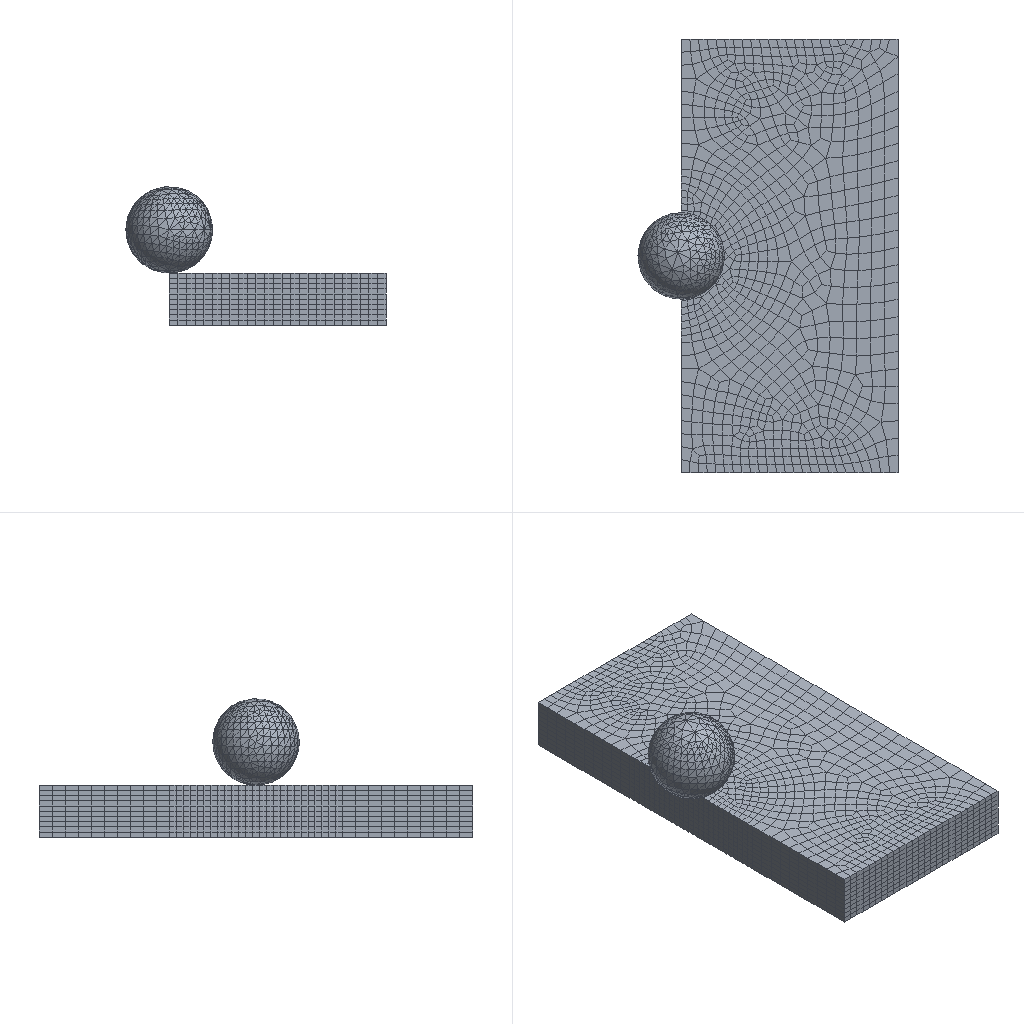Simulation study | abaqus
Set-up summary:
category,name,step,type,value,unit,region
solver,abaqus,,Abaqus/CAE 2024
units,SI m-kg-s (Pa),,inferred,E=2.078e+11 density=7800
analysis,Step-1,,dynamic explicit,nlgeom=True; time_period=4e-05
mesh,nodes,,,11335
mesh,elements,,,13296
element_type,C3D8R,,,8810
element_type,C3D4,,,4486
material,Mat-plate,,E,2.078e+11
material,Mat-plate,,nu,0.3
material,Mat-plate,,density,7800
material,Mat-plate,,yield,1.22e+09
material,Mat-plate,,behaviors,plastic; shear failure
material,Mat_ball,,E,2.09e+11
material,Mat_ball,,nu,0.3
material,Mat_ball,,density,7800
section,Mat_ball,,solid section,,,_PickedSet2
section,Mat-plate,,solid section,,,_PickedSet2
load,velocity,initial,initial condition velocity
bc,BC-plate,initial,fixed,"[dofs=rx,ry,rz,x,y,z n=6]",,_PickedSet11
bc,Symm-plate,initial,ysymm,[dofs=YSYMM],,_PickedSet12
contact,ball-plate,Step-1,contact pair,interaction=contact,,_PickedSurf9 / _PickedSet10_CNS_
constraint,rigid body,,,1
Abaqus input file, long lists of numbers shortened:
*Heading
** Job name: deck Model name: Model-1
** Generated by: Abaqus/CAE 2024
*Preprint, echo=NO, model=NO, history=NO, contact=NO
**
** PARTS
**
*Part, name=Ball
*Node
      1, 0.01545,  0.04755,           0.
      2, 0.02939, 0.04045,           0.
** (970 more lines like these left out)
*Element, type=C3D4
   1, 417, 418, 419, 420
   2, 419, 417, 421, 422
** (4484 more lines like these left out)
*Nset, nset=_PickedSet2, internal, generate
   1,  972,    1
*Elset, elset=_PickedSet2, internal, generate
    1,  4486,     1
** Section: Section-ball
*Solid Section, elset=_PickedSet2, material=Mat_ball
,
*End Part
**
*Part, name=Plate
*Node
      1,           0.,  0.1,           0.
      2,           0., -0.1,           0.
** (10360 more lines like these left out)
*Element, type=C3D8R
   1,  493,  343,   14,   13, 3331, 3181,  921,  922
   2,    2,   36,  385,   37,   61,  899, 3223,  706
** (8808 more lines like these left out)
*Nset, nset=_PickedSet2, internal, generate
     1,  10362,      1
*Elset, elset=_PickedSet2, internal, generate
    1,  8810,     1
** Section: Section-Plate
*Solid Section, elset=_PickedSet2, material=Mat-plate
,
*End Part
**
**
** ASSEMBLY
**
*Assembly, name=Assembly
**
*Instance, name=Ball-1, part=Ball
          0.,           0.,         0.11
*End Instance
**
*Instance, name=Plate-1, part=Plate
*End Instance
**
*Node
      1,           0.,           0.,  0.11
*Nset, nset=_PickedSet7, internal
 1,
*Nset, nset=_PickedSet8, internal, instance=Ball-1, generate
   1,  972,    1
*Elset, elset=_PickedSet8, internal, instance=Ball-1, generate
    1,  4486,     1
*Nset, nset=_PickedSet10, internal, instance=Plate-1
   3,   4,  79,  80,  81,  82,  83,  84,  85,  86,  87,  88,  89,  90,  91,  92
  93,  94,  95,  96,  97,  98,  99, 100, 101, 102, 103, 104, 105, 106, 107, 108
** (12 more lines like these left out)
*Elset, elset=_PickedSet10, internal, instance=Plate-1, generate
 1747,  1940,     1
*Nset, nset=_PickedSet11, internal, instance=Plate-1
    1,    2,    5,    6,    7,    8,   13,   14,   15,   16,   17,   18,   19,   20,   21,   22
   23,   24,   25,   26,   27,   28,   29,   30,   31,   32,   33,   34,   35,   36,   37,   38
** (57 more lines like these left out)
*Elset, elset=_PickedSet11, internal, instance=Plate-1
    1,    2,    3,    4,    5,    6,    7,    8,    9,   10,   11,   12,   13,   14,   15,   16
   17,   18,   19,   20,   21,   22,   23,   24,   25,   26,   27,   28,   29,   30,   31,   32
** (54 more lines like these left out)
*Nset, nset=_PickedSet12, internal, instance=Plate-1
    1,    2,    3,    4,    5,    8,    9,   12,   37,   38,   39,   40,   41,   42,   43,   44
   45,   46,   47,   48,   49,   50,   51,   52,   53,   54,   55,   56,   57,   58,   59,   60
** (30 more lines like these left out)
*Elset, elset=_PickedSet12, internal, instance=Plate-1
    2,    8,   11,   22,   23,   27,   30,   31,   33,   34,   35,   37,   38,   40,   41,   43
   44,   49,   52,   55,   60,   62,   69,   70,   84,  196,  202,  205,  216,  217,  221,  224
** (27 more lines like these left out)
*Nset, nset=_PickedSet13, internal
 1,
*Elset, elset=__PickedSurf9_S3, internal, instance=Ball-1
   19,   82,  121,  183,  188,  321,  390,  399,  417,  430,  433,  461,  489,  500,  525,  595
  624,  662,  712,  724,  725,  748,  759,  768,  815,  819,  861,  885,  946,  976, 1003, 1027
** (45 more lines like these left out)
*Elset, elset=__PickedSurf9_S4, internal, instance=Ball-1
   47,  219,  576,  610,  678,  874, 1119, 1214, 1255, 1339, 1615, 1664, 1735, 1747, 1807, 1948
 1976, 1986, 2082, 2169, 2412, 2417, 2499, 2503, 2504, 2599, 2646, 2904, 3117, 3123, 3276, 3561
** (1 more lines like these left out)
*Elset, elset=__PickedSurf9_S1, internal, instance=Ball-1
  351,  777,  783, 1037, 1132, 1137, 1529, 1583, 1886, 2555, 2673, 3428, 3594, 3846, 4419, 4421
 4470,
*Elset, elset=__PickedSurf9_S2, internal, instance=Ball-1
  521,  910, 1177, 1792, 1912, 2014, 2024, 2043, 2076, 2140, 2183, 2361, 2506, 2600, 2850, 3087
 3160, 3284, 3328, 3413, 3709, 4114
*Surface, type=ELEMENT, name=_PickedSurf9, internal
__PickedSurf9_S3, S3
__PickedSurf9_S4, S4
__PickedSurf9_S2, S2
__PickedSurf9_S1, S1
*Surface, type=NODE, name=_PickedSet10_CNS_, internal
_PickedSet10, 1.
** Constraint: Rigid-body
*Rigid Body, ref node=_PickedSet7, elset=_PickedSet8
*End Assembly
**
** MATERIALS
**
*Material, name=Mat-plate
*Density
7800.,
*Elastic
 2.078e+11, 0.3
*Plastic
 1.22e+09,0.
 2.44e+09,1.
*Shear Failure
1.0
*Material, name=Mat_ball
*Density
7800.,
*Elastic
 2.09e+11, 0.3
**
** INTERACTION PROPERTIES
**
*Surface Interaction, name=contact
**
** BOUNDARY CONDITIONS
**
** Name: BC-plate Type: Displacement/Rotation
*Boundary
_PickedSet11, 1, 1
_PickedSet11, 2, 2
_PickedSet11, 3, 3
_PickedSet11, 4, 4
_PickedSet11, 5, 5
_PickedSet11, 6, 6
** Name: Symm-plate Type: Symmetry/Antisymmetry/Encastre
*Boundary
_PickedSet12, YSYMM
**
** PREDEFINED FIELDS
**
** Name: velocity   Type: Velocity
*Initial Conditions, type=VELOCITY
_PickedSet13, 1, 800.
_PickedSet13, 2, 0.
_PickedSet13, 3, -300.
** ----------------------------------------------------------------
**
** STEP: Step-1
**
*Step, name=Step-1, nlgeom=YES
*Dynamic, Explicit
, 4e-05
*Bulk Viscosity
0.06, 1.2
**
** INTERACTIONS
**
** Interaction: ball-plate
*Contact Pair, interaction=contact, mechanical constraint=KINEMATIC, cpset=ball-plate
_PickedSurf9, _PickedSet10_CNS_
**
** OUTPUT REQUESTS
**
*Restart, write, number interval=1, time marks=NO
**
** FIELD OUTPUT: F-Output-1
**
*Output, field, variable=PRESELECT
**
** HISTORY OUTPUT: H-Output-1
**
*Output, history, variable=PRESELECT
**
** HISTORY OUTPUT: H-Output-2
**
*Output, history
*Contact Output, cpset=ball-plate, variable=ALL
*End Step
Results summary:
result,odb.job_status,,,JOB_STATUS_COMPLETED_SUCCESSFULLY,"consistent, unstated (Abaqus has no unit system)"
result,steps[0].procedure,Step-1,,"*DYNAMIC, EXPLICIT","consistent, unstated (Abaqus has no unit system)"
result,steps[0].time_period,Step-1,,4e-05,"consistent, unstated (Abaqus has no unit system)"
result,steps[0].n_frames,Step-1,,21,"consistent, unstated (Abaqus has no unit system)"
result,steps[0].last_frame.id,Step-1,,52,"consistent, unstated (Abaqus has no unit system)"
result,steps[0].last_frame.value,Step-1,,4e-05,"consistent, unstated (Abaqus has no unit system)"
result,steps[0].last_frame.description,Step-1,,Increment        52: Step Time =   4.0000E-05,"consistent, unstated (Abaqus has no unit system)"
result,steps[0].completed,Step-1,,True,"consistent, unstated (Abaqus has no unit system)"
result,steps[0].max_U_magnitude,Step-1,,0.03374,"consistent, unstated (Abaqus has no unit system)"
result,steps[0].max_S_mises,Step-1,,2.42007e+09,"consistent, unstated (Abaqus has no unit system)"
result,steps[0].RF_sum[1],Step-1,,-2.61791e+06,"consistent, unstated (Abaqus has no unit system)"
result,steps[0].RF_sum[2],Step-1,,-60001.6,"consistent, unstated (Abaqus has no unit system)"
result,steps[0].RF_sum[3],Step-1,,9.52451e+06,"consistent, unstated (Abaqus has no unit system)"
result,steps[0].diagnostic.n_increments,Step-1,,21,"consistent, unstated (Abaqus has no unit system)"